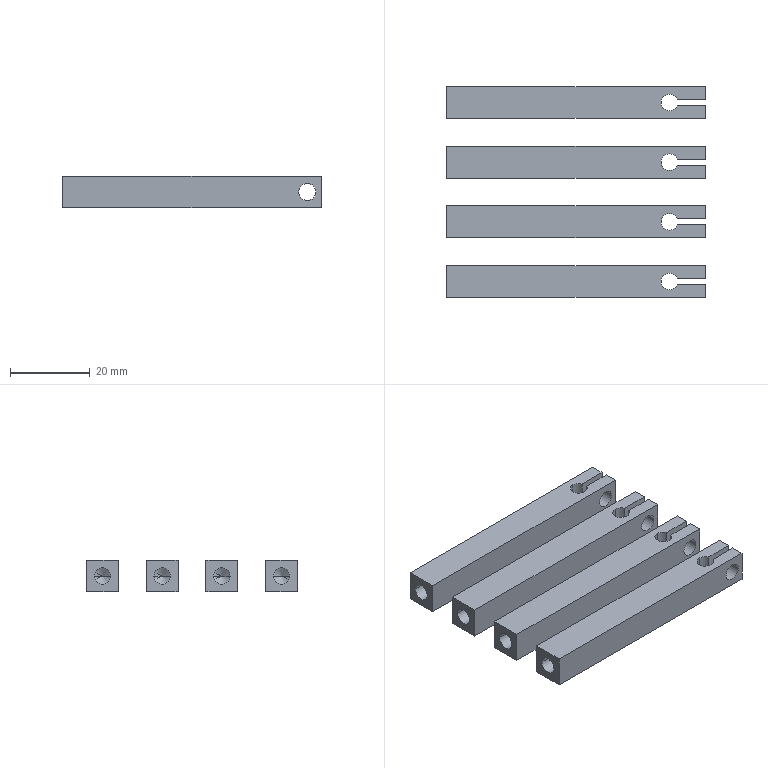NC program | NX | posted with a generic post | part box 65 x 53 x 8 mm
Lines 1 to 852 of 3458:
N10 G17 G21 G94 G90
(DRILLING , TOOL : D6A45)
N12 T07 M6
N14 G54
N16 G17 G0 G90 X-22.5 Y-23.5 B0. C0. S5000 M3
N18 G43 Z30. H7
N20 G94 G81 G98 Z-2.2 F250. R3.
N22 X-7.5
N24 X7.5
N26 X22.5
N28 G80
N30 G0 X22.5 Y-23.5 Z30.
N32 M5
(DRILLING_COPY_COPY , TOOL : 4.2ZT)
N34 T14 M6
N36 G54
N38 G17 G0 G90 X-22.5 Y-23.5 B0. C0. S2000 M3
N40 G43 Z30. H14
N42 G94 G83 G98 Z-10.762 F200. Q2. R3.
N44 X-7.5
N46 X7.5
N48 X22.5
N50 G80
N52 G0 X22.5 Y-23.5 Z30.
N54 M5
(ZLEVEL_PROFILE , TOOL : D6)
N56 T06 M6
N58 G54
N60 G17 G0 G90 X15.4 Y12.219 B0. C0. S9500 M3
N62 G43 Z30. H6
N64 Z1.5
N66 G94 G1 Y32.749 Z0.424 F1000.
N68 X15.513 Y33.365 Z0.391
N70 X15.746 Y33.945 Z0.359
N72 X16.091 Y34.467 Z0.326
N74 X16.533 Y34.909 Z0.293
N76 X17.055 Y35.254 Z0.26
N78 X17.635 Y35.487 Z0.227
N80 X18.251 Y35.6 Z0.195
N82 X26.749 Z-0.251
N84 X27.365 Y35.487 Z-0.284
N86 X27.945 Y35.254 Z-0.316
N88 X28.467 Y34.909 Z-0.349
N90 X28.909 Y34.467 Z-0.382
N92 X29.254 Y33.945 Z-0.415
N94 X29.487 Y33.365 Z-0.447
N96 X29.6 Y32.749 Z-0.48
N98 Y32.5 Z-0.493
N100 Y-32.5 F2200.
N102 G2 X26.5 Y-35.6 R3.1
N104 G1 X23.25
N106 G2 X22.5 Y-35.508 R3.1
N108 X21.75 Y-35.6 R3.1
N110 G1 X18.5
N112 G2 X15.4 Y-32.5 R3.1
N114 G1 Y32.5
N116 G2 X18.5 Y35.6 R3.1
N118 G1 X26.5
N120 G2 X29.6 Y32.5 R3.1
N122 G1 Y4.237 Z-0.987
N124 Y-32.5
N126 G2 X26.5 Y-35.6 R3.1
N128 G1 X23.25
N130 G2 X22.5 Y-35.508 R3.1
N132 X21.75 Y-35.6 R3.1
N134 G1 X18.5
N136 G2 X15.4 Y-32.5 R3.1
N138 G1 Y32.5
N140 G2 X18.5 Y35.6 R3.1
N142 G1 X26.5
N144 G2 X29.6 Y32.5 R3.1
N146 G1 Y4.237 Z-1.48
N148 Y-32.5
N150 G2 X26.5 Y-35.6 R3.1
N152 G1 X23.25
N154 G2 X22.5 Y-35.508 R3.1
N156 X21.75 Y-35.6 R3.1
N158 G1 X18.5
N160 G2 X15.4 Y-32.5 R3.1
N162 G1 Y32.5
N164 G2 X18.5 Y35.6 R3.1
N166 G1 X26.5
N168 G2 X29.6 Y32.5 R3.1
N170 G1 Y4.237 Z-1.973
N172 Y-32.5
N174 G2 X26.5 Y-35.6 R3.1
N176 G1 X23.25
N178 G2 X22.5 Y-35.508 R3.1
N180 X21.75 Y-35.6 R3.1
N182 G1 X18.5
N184 G2 X15.4 Y-32.5 R3.1
N186 G1 Y32.5
N188 G2 X18.5 Y35.6 R3.1
N190 G1 X26.5
N192 G2 X29.6 Y32.5 R3.1
N194 G1 Y4.237 Z-2.467
N196 Y-32.5
N198 G2 X26.5 Y-35.6 R3.1
N200 G1 X23.25
N202 G2 X22.5 Y-35.508 R3.1
N204 X21.75 Y-35.6 R3.1
N206 G1 X18.5
N208 G2 X15.4 Y-32.5 R3.1
N210 G1 Y32.5
N212 G2 X18.5 Y35.6 R3.1
N214 G1 X26.5
N216 G2 X29.6 Y32.5 R3.1
N218 G1 Y4.237 Z-2.96
N220 Y-32.5
N222 G2 X26.5 Y-35.6 R3.1
N224 G1 X23.25
N226 G2 X22.5 Y-35.508 R3.1
N228 X21.75 Y-35.6 R3.1
N230 G1 X18.5
N232 G2 X15.4 Y-32.5 R3.1
N234 G1 Y32.5
N236 G2 X18.5 Y35.6 R3.1
N238 G1 X26.5
N240 G2 X29.6 Y32.5 R3.1
N242 G1 Y4.237 Z-3.453
N244 Y-32.5
N246 G2 X26.5 Y-35.6 R3.1
N248 G1 X23.25
N250 G2 X22.5 Y-35.508 R3.1
N252 X21.75 Y-35.6 R3.1
N254 G1 X18.5
N256 G2 X15.4 Y-32.5 R3.1
N258 G1 Y32.5
N260 G2 X18.5 Y35.6 R3.1
N262 G1 X26.5
N264 G2 X29.6 Y32.5 R3.1
N266 G1 Y4.237 Z-3.947
N268 Y-32.5
N270 G2 X26.5 Y-35.6 R3.1
N272 G1 X23.25
N274 G2 X22.5 Y-35.508 R3.1
N276 X21.75 Y-35.6 R3.1
N278 G1 X18.5
N280 G2 X15.4 Y-32.5 R3.1
N282 G1 Y32.5
N284 G2 X18.5 Y35.6 R3.1
N286 G1 X26.5
N288 G2 X29.6 Y32.5 R3.1
N290 G1 Y4.237 Z-4.44
N292 Y-32.5
N294 G2 X26.5 Y-35.6 R3.1
N296 G1 X23.25
N298 G2 X22.5 Y-35.508 R3.1
N300 X21.75 Y-35.6 R3.1
N302 G1 X18.5
N304 G2 X15.4 Y-32.5 R3.1
N306 G1 Y32.5
N308 G2 X18.5 Y35.6 R3.1
N310 G1 X26.5
N312 G2 X29.6 Y32.5 R3.1
N314 G1 Y4.237 Z-4.933
N316 Y-32.5
N318 G2 X26.5 Y-35.6 R3.1
N320 G1 X23.25
N322 G2 X22.5 Y-35.508 R3.1
N324 X21.75 Y-35.6 R3.1
N326 G1 X18.5
N328 G2 X15.4 Y-32.5 R3.1
N330 G1 Y32.5
N332 G2 X18.5 Y35.6 R3.1
N334 G1 X26.5
N336 G2 X29.6 Y32.5 R3.1
N338 G1 Y4.237 Z-5.427
N340 Y-32.5
N342 G2 X26.5 Y-35.6 R3.1
N344 G1 X23.25
N346 G2 X22.5 Y-35.508 R3.1
N348 X21.75 Y-35.6 R3.1
N350 G1 X18.5
N352 G2 X15.4 Y-32.5 R3.1
N354 G1 Y32.5
N356 G2 X18.5 Y35.6 R3.1
N358 G1 X26.5
N360 G2 X29.6 Y32.5 R3.1
N362 G1 Y4.237 Z-5.92
N364 Y-32.5
N366 G2 X26.5 Y-35.6 R3.1
N368 G1 X23.25
N370 G2 X22.5 Y-35.508 R3.1
N372 X21.75 Y-35.6 R3.1
N374 G1 X18.5
N376 G2 X15.4 Y-32.5 R3.1
N378 G1 Y32.5
N380 G2 X18.5 Y35.6 R3.1
N382 G1 X26.5
N384 G2 X29.6 Y32.5 R3.1
N386 G1 Y4.237 Z-6.413
N388 Y-32.5
N390 G2 X26.5 Y-35.6 R3.1
N392 G1 X23.25
N394 G2 X22.5 Y-35.508 R3.1
N396 X21.75 Y-35.6 R3.1
N398 G1 X18.5
N400 G2 X15.4 Y-32.5 R3.1
N402 G1 Y32.5
N404 G2 X18.5 Y35.6 R3.1
N406 G1 X26.5
N408 G2 X29.6 Y32.5 R3.1
N410 G1 Y4.237 Z-6.907
N412 Y-32.5
N414 G2 X26.5 Y-35.6 R3.1
N416 G1 X23.25
N418 G2 X22.5 Y-35.508 R3.1
N420 X21.75 Y-35.6 R3.1
N422 G1 X18.5
N424 G2 X15.4 Y-32.5 R3.1
N426 G1 Y32.5
N428 G2 X18.5 Y35.6 R3.1
N430 G1 X26.5
N432 G2 X29.6 Y32.5 R3.1
N434 G1 Y4.237 Z-7.4
N436 Y-32.5
N438 G2 X26.5 Y-35.6 R3.1
N440 G1 X23.25
N442 G2 X22.5 Y-35.508 R3.1
N444 X21.75 Y-35.6 R3.1
N446 G1 X18.5
N448 G2 X15.4 Y-32.5 R3.1
N450 G1 Y32.5
N452 G2 X18.5 Y35.6 R3.1
N454 G1 X26.5
N456 G2 X29.6 Y32.5 R3.1
N458 G1 Y4.237
N460 Z-5.9
N462 G0 Z53.
N464 X0.4 Y12.219
N466 Z1.5
N468 G1 Y32.749 Z0.424 F1000.
N470 X0.513 Y33.365 Z0.391
N472 X0.746 Y33.945 Z0.359
N474 X1.091 Y34.467 Z0.326
N476 X1.533 Y34.909 Z0.293
N478 X2.055 Y35.254 Z0.26
N480 X2.635 Y35.487 Z0.227
N482 X3.251 Y35.6 Z0.195
N484 X11.749 Z-0.251
N486 X12.365 Y35.487 Z-0.284
N488 X12.945 Y35.254 Z-0.316
N490 X13.467 Y34.909 Z-0.349
N492 X13.909 Y34.467 Z-0.382
N494 X14.254 Y33.945 Z-0.415
N496 X14.487 Y33.365 Z-0.447
N498 X14.6 Y32.749 Z-0.48
N500 Y32.5 Z-0.493
N502 Y-32.5 F2200.
N504 G2 X11.5 Y-35.6 R3.1
N506 G1 X8.25
N508 G2 X7.5 Y-35.508 R3.1
N510 X6.75 Y-35.6 R3.1
N512 G1 X3.5
N514 G2 X0.4 Y-32.5 R3.1
N516 G1 Y32.5
N518 G2 X3.5 Y35.6 R3.1
N520 G1 X11.5
N522 G2 X14.6 Y32.5 R3.1
N524 G1 Y4.237 Z-0.987
N526 Y-32.5
N528 G2 X11.5 Y-35.6 R3.1
N530 G1 X8.25
N532 G2 X7.5 Y-35.508 R3.1
N534 X6.75 Y-35.6 R3.1
N536 G1 X3.5
N538 G2 X0.4 Y-32.5 R3.1
N540 G1 Y32.5
N542 G2 X3.5 Y35.6 R3.1
N544 G1 X11.5
N546 G2 X14.6 Y32.5 R3.1
N548 G1 Y4.237 Z-1.48
N550 Y-32.5
N552 G2 X11.5 Y-35.6 R3.1
N554 G1 X8.25
N556 G2 X7.5 Y-35.508 R3.1
N558 X6.75 Y-35.6 R3.1
N560 G1 X3.5
N562 G2 X0.4 Y-32.5 R3.1
N564 G1 Y32.5
N566 G2 X3.5 Y35.6 R3.1
N568 G1 X11.5
N570 G2 X14.6 Y32.5 R3.1
N572 G1 Y4.237 Z-1.973
N574 Y-32.5
N576 G2 X11.5 Y-35.6 R3.1
N578 G1 X8.25
N580 G2 X7.5 Y-35.508 R3.1
N582 X6.75 Y-35.6 R3.1
N584 G1 X3.5
N586 G2 X0.4 Y-32.5 R3.1
N588 G1 Y32.5
N590 G2 X3.5 Y35.6 R3.1
N592 G1 X11.5
N594 G2 X14.6 Y32.5 R3.1
N596 G1 Y4.237 Z-2.467
N598 Y-32.5
N600 G2 X11.5 Y-35.6 R3.1
N602 G1 X8.25
N604 G2 X7.5 Y-35.508 R3.1
N606 X6.75 Y-35.6 R3.1
N608 G1 X3.5
N610 G2 X0.4 Y-32.5 R3.1
N612 G1 Y32.5
N614 G2 X3.5 Y35.6 R3.1
N616 G1 X11.5
N618 G2 X14.6 Y32.5 R3.1
N620 G1 Y4.237 Z-2.96
N622 Y-32.5
N624 G2 X11.5 Y-35.6 R3.1
N626 G1 X8.25
N628 G2 X7.5 Y-35.508 R3.1
N630 X6.75 Y-35.6 R3.1
N632 G1 X3.5
N634 G2 X0.4 Y-32.5 R3.1
N636 G1 Y32.5
N638 G2 X3.5 Y35.6 R3.1
N640 G1 X11.5
N642 G2 X14.6 Y32.5 R3.1
N644 G1 Y4.237 Z-3.453
N646 Y-32.5
N648 G2 X11.5 Y-35.6 R3.1
N650 G1 X8.25
N652 G2 X7.5 Y-35.508 R3.1
N654 X6.75 Y-35.6 R3.1
N656 G1 X3.5
N658 G2 X0.4 Y-32.5 R3.1
N660 G1 Y32.5
N662 G2 X3.5 Y35.6 R3.1
N664 G1 X11.5
N666 G2 X14.6 Y32.5 R3.1
N668 G1 Y4.237 Z-3.947
N670 Y-32.5
N672 G2 X11.5 Y-35.6 R3.1
N674 G1 X8.25
N676 G2 X7.5 Y-35.508 R3.1
N678 X6.75 Y-35.6 R3.1
N680 G1 X3.5
N682 G2 X0.4 Y-32.5 R3.1
N684 G1 Y32.5
N686 G2 X3.5 Y35.6 R3.1
N688 G1 X11.5
N690 G2 X14.6 Y32.5 R3.1
N692 G1 Y4.237 Z-4.44
N694 Y-32.5
N696 G2 X11.5 Y-35.6 R3.1
N698 G1 X8.25
N700 G2 X7.5 Y-35.508 R3.1
N702 X6.75 Y-35.6 R3.1
N704 G1 X3.5
N706 G2 X0.4 Y-32.5 R3.1
N708 G1 Y32.5
N710 G2 X3.5 Y35.6 R3.1
N712 G1 X11.5
N714 G2 X14.6 Y32.5 R3.1
N716 G1 Y4.237 Z-4.933
N718 Y-32.5
N720 G2 X11.5 Y-35.6 R3.1
N722 G1 X8.25
N724 G2 X7.5 Y-35.508 R3.1
N726 X6.75 Y-35.6 R3.1
N728 G1 X3.5
N730 G2 X0.4 Y-32.5 R3.1
N732 G1 Y32.5
N734 G2 X3.5 Y35.6 R3.1
N736 G1 X11.5
N738 G2 X14.6 Y32.5 R3.1
N740 G1 Y4.237 Z-5.427
N742 Y-32.5
N744 G2 X11.5 Y-35.6 R3.1
N746 G1 X8.25
N748 G2 X7.5 Y-35.508 R3.1
N750 X6.75 Y-35.6 R3.1
N752 G1 X3.5
N754 G2 X0.4 Y-32.5 R3.1
N756 G1 Y32.5
N758 G2 X3.5 Y35.6 R3.1
N760 G1 X11.5
N762 G2 X14.6 Y32.5 R3.1
N764 G1 Y4.237 Z-5.92
N766 Y-32.5
N768 G2 X11.5 Y-35.6 R3.1
N770 G1 X8.25
N772 G2 X7.5 Y-35.508 R3.1
N774 X6.75 Y-35.6 R3.1
N776 G1 X3.5
N778 G2 X0.4 Y-32.5 R3.1
N780 G1 Y32.5
N782 G2 X3.5 Y35.6 R3.1
N784 G1 X11.5
N786 G2 X14.6 Y32.5 R3.1
N788 G1 Y4.237 Z-6.413
N790 Y-32.5
N792 G2 X11.5 Y-35.6 R3.1
N794 G1 X8.25
N796 G2 X7.5 Y-35.508 R3.1
N798 X6.75 Y-35.6 R3.1
N800 G1 X3.5
N802 G2 X0.4 Y-32.5 R3.1
N804 G1 Y32.5
N806 G2 X3.5 Y35.6 R3.1
N808 G1 X11.5
N810 G2 X14.6 Y32.5 R3.1
N812 G1 Y4.237 Z-6.907
N814 Y-32.5
N816 G2 X11.5 Y-35.6 R3.1
N818 G1 X8.25
N820 G2 X7.5 Y-35.508 R3.1
N822 X6.75 Y-35.6 R3.1
N824 G1 X3.5
N826 G2 X0.4 Y-32.5 R3.1
N828 G1 Y32.5
N830 G2 X3.5 Y35.6 R3.1
N832 G1 X11.5
N834 G2 X14.6 Y32.5 R3.1
N836 G1 Y4.237 Z-7.4
N838 Y-32.5
N840 G2 X11.5 Y-35.6 R3.1
N842 G1 X8.25
N844 G2 X7.5 Y-35.508 R3.1
N846 X6.75 Y-35.6 R3.1
N848 G1 X3.5
N850 G2 X0.4 Y-32.5 R3.1
N852 G1 Y32.5
N854 G2 X3.5 Y35.6 R3.1
N856 G1 X11.5
N858 G2 X14.6 Y32.5 R3.1
N860 G1 Y4.237
N862 Z-5.9
N864 G0 Z53.
N866 X-15.4 Y-12.238
N868 Z1.5
N870 G1 Y-32.749 Z0.425 F1000.
N872 X-15.513 Y-33.365 Z0.392
N874 X-15.746 Y-33.945 Z0.359
N876 X-16.091 Y-34.467 Z0.327
N878 X-16.533 Y-34.909 Z0.294
N880 X-17.055 Y-35.254 Z0.261
N882 X-17.635 Y-35.487 Z0.228
N884 X-18.251 Y-35.6 Z0.196
N886 X-21.999 Z-0.001
N888 X-22.258 Y-35.568 Z-0.015
N890 X-22.5 Y-35.508 Z-0.028
N892 X-22.742 Y-35.568 Z-0.041
N894 X-23.001 Y-35.6 Z-0.054
N896 X-26.749 Z-0.251
N898 X-27.365 Y-35.487 Z-0.284
N900 X-27.945 Y-35.254 Z-0.316
N902 X-28.467 Y-34.909 Z-0.349
N904 X-28.909 Y-34.467 Z-0.382
N906 X-29.254 Y-33.945 Z-0.415
N908 X-29.487 Y-33.365 Z-0.447
N910 X-29.6 Y-32.749 Z-0.48
N912 Y-32.5 Z-0.493
N914 Y32.5 F2200.
N916 G2 X-26.5 Y35.6 R3.1
N918 G1 X-18.5
N920 G2 X-15.4 Y32.5 R3.1
N922 G1 Y-32.5
N924 G2 X-18.5 Y-35.6 R3.1
N926 G1 X-21.75
N928 G2 X-22.5 Y-35.508 R3.1
N930 X-23.25 Y-35.6 R3.1
N932 G1 X-26.5
N934 G2 X-29.6 Y-32.5 R3.1
N936 G1 Y-4.237 Z-0.987
N938 Y32.5
N940 G2 X-26.5 Y35.6 R3.1
N942 G1 X-18.5
N944 G2 X-15.4 Y32.5 R3.1
N946 G1 Y-32.5
N948 G2 X-18.5 Y-35.6 R3.1
N950 G1 X-21.75
N952 G2 X-22.5 Y-35.508 R3.1
N954 X-23.25 Y-35.6 R3.1
N956 G1 X-26.5
N958 G2 X-29.6 Y-32.5 R3.1
N960 G1 Y-4.237 Z-1.48
N962 Y32.5
N964 G2 X-26.5 Y35.6 R3.1
N966 G1 X-18.5
N968 G2 X-15.4 Y32.5 R3.1
N970 G1 Y-32.5
N972 G2 X-18.5 Y-35.6 R3.1
N974 G1 X-21.75
N976 G2 X-22.5 Y-35.508 R3.1
N978 X-23.25 Y-35.6 R3.1
N980 G1 X-26.5
N982 G2 X-29.6 Y-32.5 R3.1
N984 G1 Y-4.237 Z-1.973
N986 Y32.5
N988 G2 X-26.5 Y35.6 R3.1
N990 G1 X-18.5
N992 G2 X-15.4 Y32.5 R3.1
N994 G1 Y-32.5
N996 G2 X-18.5 Y-35.6 R3.1
N998 G1 X-21.75
N1000 G2 X-22.5 Y-35.508 R3.1
N1002 X-23.25 Y-35.6 R3.1
N1004 G1 X-26.5
N1006 G2 X-29.6 Y-32.5 R3.1
N1008 G1 Y-4.237 Z-2.467
N1010 Y32.5
N1012 G2 X-26.5 Y35.6 R3.1
N1014 G1 X-18.5
N1016 G2 X-15.4 Y32.5 R3.1
N1018 G1 Y-32.5
N1020 G2 X-18.5 Y-35.6 R3.1
N1022 G1 X-21.75
N1024 G2 X-22.5 Y-35.508 R3.1
N1026 X-23.25 Y-35.6 R3.1
N1028 G1 X-26.5
N1030 G2 X-29.6 Y-32.5 R3.1
N1032 G1 Y-4.237 Z-2.96
N1034 Y32.5
N1036 G2 X-26.5 Y35.6 R3.1
N1038 G1 X-18.5
N1040 G2 X-15.4 Y32.5 R3.1
N1042 G1 Y-32.5
N1044 G2 X-18.5 Y-35.6 R3.1
N1046 G1 X-21.75
N1048 G2 X-22.5 Y-35.508 R3.1
N1050 X-23.25 Y-35.6 R3.1
N1052 G1 X-26.5
N1054 G2 X-29.6 Y-32.5 R3.1
N1056 G1 Y-4.237 Z-3.453
N1058 Y32.5
N1060 G2 X-26.5 Y35.6 R3.1
N1062 G1 X-18.5
N1064 G2 X-15.4 Y32.5 R3.1
N1066 G1 Y-32.5
N1068 G2 X-18.5 Y-35.6 R3.1
N1070 G1 X-21.75
N1072 G2 X-22.5 Y-35.508 R3.1
N1074 X-23.25 Y-35.6 R3.1
N1076 G1 X-26.5
N1078 G2 X-29.6 Y-32.5 R3.1
N1080 G1 Y-4.237 Z-3.947
N1082 Y32.5
N1084 G2 X-26.5 Y35.6 R3.1
N1086 G1 X-18.5
N1088 G2 X-15.4 Y32.5 R3.1
N1090 G1 Y-32.5
N1092 G2 X-18.5 Y-35.6 R3.1
N1094 G1 X-21.75
N1096 G2 X-22.5 Y-35.508 R3.1
N1098 X-23.25 Y-35.6 R3.1
N1100 G1 X-26.5
N1102 G2 X-29.6 Y-32.5 R3.1
N1104 G1 Y-4.237 Z-4.44
N1106 Y32.5
N1108 G2 X-26.5 Y35.6 R3.1
N1110 G1 X-18.5
N1112 G2 X-15.4 Y32.5 R3.1
N1114 G1 Y-32.5
N1116 G2 X-18.5 Y-35.6 R3.1
N1118 G1 X-21.75
N1120 G2 X-22.5 Y-35.508 R3.1
N1122 X-23.25 Y-35.6 R3.1
N1124 G1 X-26.5
N1126 G2 X-29.6 Y-32.5 R3.1
N1128 G1 Y-4.237 Z-4.933
N1130 Y32.5
N1132 G2 X-26.5 Y35.6 R3.1
N1134 G1 X-18.5
N1136 G2 X-15.4 Y32.5 R3.1
N1138 G1 Y-32.5
N1140 G2 X-18.5 Y-35.6 R3.1
N1142 G1 X-21.75
N1144 G2 X-22.5 Y-35.508 R3.1
N1146 X-23.25 Y-35.6 R3.1
N1148 G1 X-26.5
N1150 G2 X-29.6 Y-32.5 R3.1
N1152 G1 Y-4.237 Z-5.427
N1154 Y32.5
N1156 G2 X-26.5 Y35.6 R3.1
N1158 G1 X-18.5
N1160 G2 X-15.4 Y32.5 R3.1
N1162 G1 Y-32.5
N1164 G2 X-18.5 Y-35.6 R3.1
N1166 G1 X-21.75
N1168 G2 X-22.5 Y-35.508 R3.1
N1170 X-23.25 Y-35.6 R3.1
N1172 G1 X-26.5
N1174 G2 X-29.6 Y-32.5 R3.1
N1176 G1 Y-4.237 Z-5.92
N1178 Y32.5
N1180 G2 X-26.5 Y35.6 R3.1
N1182 G1 X-18.5
N1184 G2 X-15.4 Y32.5 R3.1
N1186 G1 Y-32.5
N1188 G2 X-18.5 Y-35.6 R3.1
N1190 G1 X-21.75
N1192 G2 X-22.5 Y-35.508 R3.1
N1194 X-23.25 Y-35.6 R3.1
N1196 G1 X-26.5
N1198 G2 X-29.6 Y-32.5 R3.1
N1200 G1 Y-4.237 Z-6.413
N1202 Y32.5
N1204 G2 X-26.5 Y35.6 R3.1
N1206 G1 X-18.5
N1208 G2 X-15.4 Y32.5 R3.1
N1210 G1 Y-32.5
N1212 G2 X-18.5 Y-35.6 R3.1
N1214 G1 X-21.75
N1216 G2 X-22.5 Y-35.508 R3.1
N1218 X-23.25 Y-35.6 R3.1
N1220 G1 X-26.5
N1222 G2 X-29.6 Y-32.5 R3.1
N1224 G1 Y-4.237 Z-6.907
N1226 Y32.5
N1228 G2 X-26.5 Y35.6 R3.1
N1230 G1 X-18.5
N1232 G2 X-15.4 Y32.5 R3.1
N1234 G1 Y-32.5
N1236 G2 X-18.5 Y-35.6 R3.1
N1238 G1 X-21.75
N1240 G2 X-22.5 Y-35.508 R3.1
N1242 X-23.25 Y-35.6 R3.1
N1244 G1 X-26.5
N1246 G2 X-29.6 Y-32.5 R3.1
N1248 G1 Y-4.237 Z-7.4
N1250 Y32.5
N1252 G2 X-26.5 Y35.6 R3.1
N1254 G1 X-18.5
N1256 G2 X-15.4 Y32.5 R3.1
N1258 G1 Y-32.5
N1260 G2 X-18.5 Y-35.6 R3.1
N1262 G1 X-21.75
N1264 G2 X-22.5 Y-35.508 R3.1
N1266 X-23.25 Y-35.6 R3.1
N1268 G1 X-26.5
N1270 G2 X-29.6 Y-32.5 R3.1
N1272 G1 Y-4.237
N1274 Z-5.9
N1276 G0 Z53.
N1278 X-0.4 Y-12.238
N1280 Z1.5
N1282 G1 Y-32.749 Z0.425 F1000.
N1284 X-0.513 Y-33.365 Z0.392
N1286 X-0.746 Y-33.945 Z0.359
N1288 X-1.091 Y-34.467 Z0.327
N1290 X-1.533 Y-34.909 Z0.294
N1292 X-2.055 Y-35.254 Z0.261
N1294 X-2.635 Y-35.487 Z0.228
N1296 X-3.251 Y-35.6 Z0.196
N1298 X-6.999 Z-0.001
N1300 X-7.258 Y-35.568 Z-0.015
N1302 X-7.5 Y-35.508 Z-0.028
N1304 X-7.742 Y-35.568 Z-0.041
N1306 X-8.001 Y-35.6 Z-0.054
N1308 X-11.749 Z-0.251
N1310 X-12.365 Y-35.487 Z-0.284
N1312 X-12.945 Y-35.254 Z-0.316
N1314 X-13.467 Y-34.909 Z-0.349
N1316 X-13.909 Y-34.467 Z-0.382
N1318 X-14.254 Y-33.945 Z-0.415
N1320 X-14.487 Y-33.365 Z-0.447
N1322 X-14.6 Y-32.749 Z-0.48
N1324 Y-32.5 Z-0.493
N1326 Y32.5 F2200.
N1328 G2 X-11.5 Y35.6 R3.1
N1330 G1 X-3.5
N1332 G2 X-0.4 Y32.5 R3.1
N1334 G1 Y-32.5
N1336 G2 X-3.5 Y-35.6 R3.1
N1338 G1 X-6.75
N1340 G2 X-7.5 Y-35.508 R3.1
N1342 X-8.25 Y-35.6 R3.1
N1344 G1 X-11.5
N1346 G2 X-14.6 Y-32.5 R3.1
N1348 G1 Y-4.237 Z-0.987
N1350 Y32.5
N1352 G2 X-11.5 Y35.6 R3.1
N1354 G1 X-3.5
N1356 G2 X-0.4 Y32.5 R3.1
N1358 G1 Y-32.5
N1360 G2 X-3.5 Y-35.6 R3.1
N1362 G1 X-6.75
N1364 G2 X-7.5 Y-35.508 R3.1
N1366 X-8.25 Y-35.6 R3.1
N1368 G1 X-11.5
N1370 G2 X-14.6 Y-32.5 R3.1
N1372 G1 Y-4.237 Z-1.48
N1374 Y32.5
N1376 G2 X-11.5 Y35.6 R3.1
N1378 G1 X-3.5
N1380 G2 X-0.4 Y32.5 R3.1
N1382 G1 Y-32.5
N1384 G2 X-3.5 Y-35.6 R3.1
N1386 G1 X-6.75
N1388 G2 X-7.5 Y-35.508 R3.1
N1390 X-8.25 Y-35.6 R3.1
N1392 G1 X-11.5
N1394 G2 X-14.6 Y-32.5 R3.1
N1396 G1 Y-4.237 Z-1.973
N1398 Y32.5
N1400 G2 X-11.5 Y35.6 R3.1
N1402 G1 X-3.5
N1404 G2 X-0.4 Y32.5 R3.1
N1406 G1 Y-32.5
N1408 G2 X-3.5 Y-35.6 R3.1
N1410 G1 X-6.75
N1412 G2 X-7.5 Y-35.508 R3.1
N1414 X-8.25 Y-35.6 R3.1
N1416 G1 X-11.5
N1418 G2 X-14.6 Y-32.5 R3.1
N1420 G1 Y-4.237 Z-2.467
N1422 Y32.5
N1424 G2 X-11.5 Y35.6 R3.1
N1426 G1 X-3.5
N1428 G2 X-0.4 Y32.5 R3.1
N1430 G1 Y-32.5
N1432 G2 X-3.5 Y-35.6 R3.1
N1434 G1 X-6.75
N1436 G2 X-7.5 Y-35.508 R3.1
N1438 X-8.25 Y-35.6 R3.1
N1440 G1 X-11.5
N1442 G2 X-14.6 Y-32.5 R3.1
N1444 G1 Y-4.237 Z-2.96
N1446 Y32.5
N1448 G2 X-11.5 Y35.6 R3.1
N1450 G1 X-3.5
N1452 G2 X-0.4 Y32.5 R3.1
N1454 G1 Y-32.5
N1456 G2 X-3.5 Y-35.6 R3.1
N1458 G1 X-6.75
N1460 G2 X-7.5 Y-35.508 R3.1
N1462 X-8.25 Y-35.6 R3.1
N1464 G1 X-11.5
N1466 G2 X-14.6 Y-32.5 R3.1
N1468 G1 Y-4.237 Z-3.453
N1470 Y32.5
N1472 G2 X-11.5 Y35.6 R3.1
N1474 G1 X-3.5
N1476 G2 X-0.4 Y32.5 R3.1
N1478 G1 Y-32.5
N1480 G2 X-3.5 Y-35.6 R3.1
N1482 G1 X-6.75
N1484 G2 X-7.5 Y-35.508 R3.1
N1486 X-8.25 Y-35.6 R3.1
N1488 G1 X-11.5
N1490 G2 X-14.6 Y-32.5 R3.1
N1492 G1 Y-4.237 Z-3.947
N1494 Y32.5
N1496 G2 X-11.5 Y35.6 R3.1
N1498 G1 X-3.5
N1500 G2 X-0.4 Y32.5 R3.1
N1502 G1 Y-32.5
N1504 G2 X-3.5 Y-35.6 R3.1
N1506 G1 X-6.75
N1508 G2 X-7.5 Y-35.508 R3.1
N1510 X-8.25 Y-35.6 R3.1
N1512 G1 X-11.5
N1514 G2 X-14.6 Y-32.5 R3.1
N1516 G1 Y-4.237 Z-4.44
N1518 Y32.5
N1520 G2 X-11.5 Y35.6 R3.1
N1522 G1 X-3.5
N1524 G2 X-0.4 Y32.5 R3.1
N1526 G1 Y-32.5
N1528 G2 X-3.5 Y-35.6 R3.1
N1530 G1 X-6.75
N1532 G2 X-7.5 Y-35.508 R3.1
N1534 X-8.25 Y-35.6 R3.1
N1536 G1 X-11.5
N1538 G2 X-14.6 Y-32.5 R3.1
N1540 G1 Y-4.237 Z-4.933
N1542 Y32.5
N1544 G2 X-11.5 Y35.6 R3.1
N1546 G1 X-3.5
N1548 G2 X-0.4 Y32.5 R3.1
N1550 G1 Y-32.5
N1552 G2 X-3.5 Y-35.6 R3.1
N1554 G1 X-6.75
N1556 G2 X-7.5 Y-35.508 R3.1
N1558 X-8.25 Y-35.6 R3.1
N1560 G1 X-11.5
N1562 G2 X-14.6 Y-32.5 R3.1
N1564 G1 Y-4.237 Z-5.427
N1566 Y32.5
N1568 G2 X-11.5 Y35.6 R3.1
N1570 G1 X-3.5
N1572 G2 X-0.4 Y32.5 R3.1
N1574 G1 Y-32.5
N1576 G2 X-3.5 Y-35.6 R3.1
N1578 G1 X-6.75
N1580 G2 X-7.5 Y-35.508 R3.1
N1582 X-8.25 Y-35.6 R3.1
N1584 G1 X-11.5
N1586 G2 X-14.6 Y-32.5 R3.1
N1588 G1 Y-4.237 Z-5.92
N1590 Y32.5
N1592 G2 X-11.5 Y35.6 R3.1
N1594 G1 X-3.5
N1596 G2 X-0.4 Y32.5 R3.1
N1598 G1 Y-32.5
N1600 G2 X-3.5 Y-35.6 R3.1
N1602 G1 X-6.75
N1604 G2 X-7.5 Y-35.508 R3.1
N1606 X-8.25 Y-35.6 R3.1
N1608 G1 X-11.5
N1610 G2 X-14.6 Y-32.5 R3.1
N1612 G1 Y-4.237 Z-6.413
N1614 Y32.5
N1616 G2 X-11.5 Y35.6 R3.1
N1618 G1 X-3.5
N1620 G2 X-0.4 Y32.5 R3.1
N1622 G1 Y-32.5
N1624 G2 X-3.5 Y-35.6 R3.1
N1626 G1 X-6.75
N1628 G2 X-7.5 Y-35.508 R3.1
N1630 X-8.25 Y-35.6 R3.1
N1632 G1 X-11.5
N1634 G2 X-14.6 Y-32.5 R3.1
N1636 G1 Y-4.237 Z-6.907
N1638 Y32.5
N1640 G2 X-11.5 Y35.6 R3.1
N1642 G1 X-3.5
N1644 G2 X-0.4 Y32.5 R3.1
N1646 G1 Y-32.5
N1648 G2 X-3.5 Y-35.6 R3.1
N1650 G1 X-6.75
N1652 G2 X-7.5 Y-35.508 R3.1
N1654 X-8.25 Y-35.6 R3.1
N1656 G1 X-11.5
N1658 G2 X-14.6 Y-32.5 R3.1
N1660 G1 Y-4.237 Z-7.4
N1662 Y32.5
N1664 G2 X-11.5 Y35.6 R3.1
N1666 G1 X-3.5
N1668 G2 X-0.4 Y32.5 R3.1
N1670 G1 Y-32.5
N1672 G2 X-3.5 Y-35.6 R3.1
N1674 G1 X-6.75
N1676 G2 X-7.5 Y-35.508 R3.1
N1678 X-8.25 Y-35.6 R3.1
N1680 G1 X-11.5
N1682 G2 X-14.6 Y-32.5 R3.1
N1684 G1 Y-4.237
N1686 Z-5.9
N1688 G0 Z30.
N1690 M5